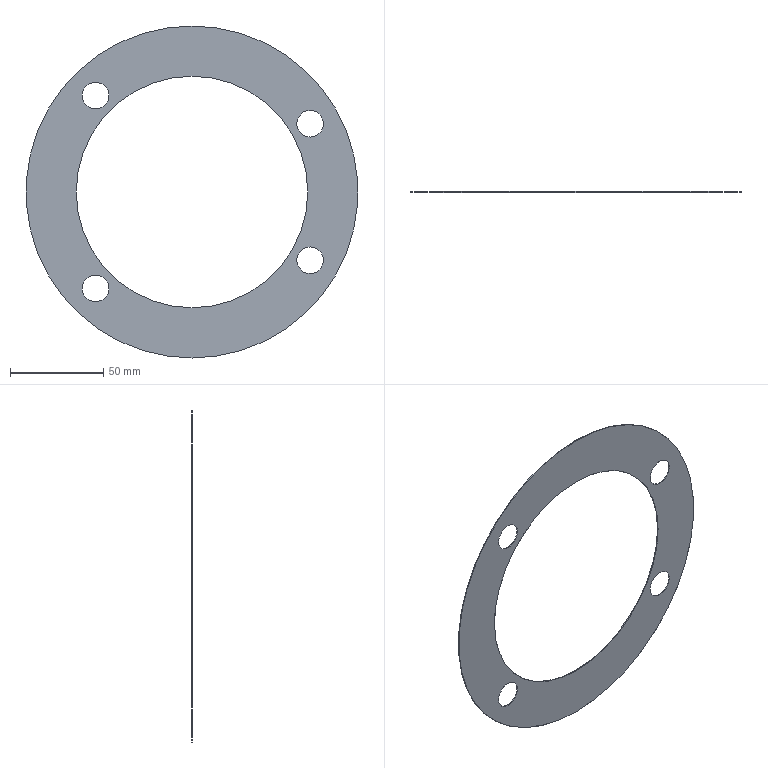Part | SolidWorks | features 3DProfileFeature 1, Extrusion 1, HoleWzd 1, MirrorPattern 1 | 1 solid | 14 faces | box 177.8 x 0.381 x 177.8 mm | volume 4618 mm3 | cylinder 12 | plane 2 | commonest cylinder face diameters 14.287 x8 123.95 x2 177.8 x2
STEP:
#1=CARTESIAN_POINT('',(-51.638,0.,44.496));
#2=VERTEX_POINT('',#1);
#3=CARTESIAN_POINT('',(-51.638,0.,58.784));
#4=VERTEX_POINT('',#3);
#5=CARTESIAN_POINT('',(-51.638,0.,51.64));
#6=DIRECTION('',(0.,1.,0.));
#7=DIRECTION('',(0.,0.,1.));
#8=AXIS2_PLACEMENT_3D('',#5,#6,#7);
#9=CIRCLE('',#8,7.144);
#10=EDGE_CURVE('',#2,#4,#9,.T.);
#11=ORIENTED_EDGE('',*,*,#10,.F.);
#12=CARTESIAN_POINT('',(-51.638,0.381,44.496));
#13=VERTEX_POINT('',#12);
#14=CARTESIAN_POINT('',(-51.638,0.381,44.496));
#15=DIRECTION('',(0.,1.,0.));
#16=VECTOR('',#15,1000.);
#17=LINE('',#14,#16);
#18=EDGE_CURVE('',#2,#13,#17,.T.);
#19=ORIENTED_EDGE('',*,*,#18,.T.);
#20=CARTESIAN_POINT('',(-51.638,0.381,58.784));
#21=VERTEX_POINT('',#20);
#22=CARTESIAN_POINT('',(-51.638,0.381,51.64));
#23=DIRECTION('',(0.,1.,0.));
#24=DIRECTION('',(0.,0.,1.));
#25=AXIS2_PLACEMENT_3D('',#22,#23,#24);
#26=CIRCLE('',#25,7.144);
#27=EDGE_CURVE('',#13,#21,#26,.T.);
#28=ORIENTED_EDGE('',*,*,#27,.T.);
#29=CARTESIAN_POINT('',(-51.638,0.381,58.784));
#30=DIRECTION('',(0.,1.,0.));
#31=VECTOR('',#30,1000.);
#32=LINE('',#29,#31);
#33=EDGE_CURVE('',#4,#21,#32,.T.);
#34=ORIENTED_EDGE('',*,*,#33,.F.);
#35=EDGE_LOOP('',(#11,#19,#28,#34));
#36=FACE_OUTER_BOUND('',#35,.T.);
#37=CARTESIAN_POINT('',(-51.638,0.381,51.64));
#38=DIRECTION('',(0.,1.,0.));
#39=DIRECTION('',(0.,0.,1.));
#40=AXIS2_PLACEMENT_3D('',#37,#38,#39);
#41=CYLINDRICAL_SURFACE('',#40,7.144);
#42=ADVANCED_FACE('',(#36),#41,.F.);
#43=CARTESIAN_POINT('',(63.246,0.,-43.674));
#44=VERTEX_POINT('',#43);
#45=CARTESIAN_POINT('',(63.246,0.,-29.386));
#46=VERTEX_POINT('',#45);
#47=CARTESIAN_POINT('',(63.246,0.,-36.53));
#48=DIRECTION('',(0.,1.,0.));
#49=DIRECTION('',(0.,0.,1.));
#50=AXIS2_PLACEMENT_3D('',#47,#48,#49);
#51=CIRCLE('',#50,7.144);
#52=EDGE_CURVE('',#44,#46,#51,.T.);
#53=ORIENTED_EDGE('',*,*,#52,.F.);
#54=CARTESIAN_POINT('',(63.246,0.381,-43.674));
#55=VERTEX_POINT('',#54);
#56=CARTESIAN_POINT('',(63.246,0.381,-43.674));
#57=DIRECTION('',(0.,1.,0.));
#58=VECTOR('',#57,1000.);
#59=LINE('',#56,#58);
#60=EDGE_CURVE('',#44,#55,#59,.T.);
#61=ORIENTED_EDGE('',*,*,#60,.T.);
#62=CARTESIAN_POINT('',(63.246,0.381,-29.386));
#63=VERTEX_POINT('',#62);
#64=CARTESIAN_POINT('',(63.246,0.381,-36.53));
#65=DIRECTION('',(0.,1.,0.));
#66=DIRECTION('',(0.,0.,1.));
#67=AXIS2_PLACEMENT_3D('',#64,#65,#66);
#68=CIRCLE('',#67,7.144);
#69=EDGE_CURVE('',#55,#63,#68,.T.);
#70=ORIENTED_EDGE('',*,*,#69,.T.);
#71=CARTESIAN_POINT('',(63.246,0.381,-29.386));
#72=DIRECTION('',(0.,1.,0.));
#73=VECTOR('',#72,1000.);
#74=LINE('',#71,#73);
#75=EDGE_CURVE('',#46,#63,#74,.T.);
#76=ORIENTED_EDGE('',*,*,#75,.F.);
#77=EDGE_LOOP('',(#53,#61,#70,#76));
#78=FACE_OUTER_BOUND('',#77,.T.);
#79=CARTESIAN_POINT('',(63.246,0.381,-36.53));
#80=DIRECTION('',(0.,1.,0.));
#81=DIRECTION('',(0.,0.,1.));
#82=AXIS2_PLACEMENT_3D('',#79,#80,#81);
#83=CYLINDRICAL_SURFACE('',#82,7.144);
#84=ADVANCED_FACE('',(#78),#83,.F.);
#85=CARTESIAN_POINT('',(-51.638,0.,-58.784));
#86=VERTEX_POINT('',#85);
#87=CARTESIAN_POINT('',(-51.638,0.,-44.496));
#88=VERTEX_POINT('',#87);
#89=CARTESIAN_POINT('',(-51.638,0.,-51.64));
#90=DIRECTION('',(0.,1.,0.));
#91=DIRECTION('',(0.,0.,1.));
#92=AXIS2_PLACEMENT_3D('',#89,#90,#91);
#93=CIRCLE('',#92,7.144);
#94=EDGE_CURVE('',#86,#88,#93,.T.);
#95=ORIENTED_EDGE('',*,*,#94,.F.);
#96=CARTESIAN_POINT('',(-51.638,0.381,-58.784));
#97=VERTEX_POINT('',#96);
#98=CARTESIAN_POINT('',(-51.638,0.381,-58.784));
#99=DIRECTION('',(0.,1.,0.));
#100=VECTOR('',#99,1000.);
#101=LINE('',#98,#100);
#102=EDGE_CURVE('',#86,#97,#101,.T.);
#103=ORIENTED_EDGE('',*,*,#102,.T.);
#104=CARTESIAN_POINT('',(-51.638,0.381,-44.496));
#105=VERTEX_POINT('',#104);
#106=CARTESIAN_POINT('',(-51.638,0.381,-51.64));
#107=DIRECTION('',(0.,1.,0.));
#108=DIRECTION('',(0.,0.,1.));
#109=AXIS2_PLACEMENT_3D('',#106,#107,#108);
#110=CIRCLE('',#109,7.144);
#111=EDGE_CURVE('',#97,#105,#110,.T.);
#112=ORIENTED_EDGE('',*,*,#111,.T.);
#113=CARTESIAN_POINT('',(-51.638,0.381,-44.496));
#114=DIRECTION('',(0.,1.,0.));
#115=VECTOR('',#114,1000.);
#116=LINE('',#113,#115);
#117=EDGE_CURVE('',#88,#105,#116,.T.);
#118=ORIENTED_EDGE('',*,*,#117,.F.);
#119=EDGE_LOOP('',(#95,#103,#112,#118));
#120=FACE_OUTER_BOUND('',#119,.T.);
#121=CARTESIAN_POINT('',(-51.638,0.381,-51.64));
#122=DIRECTION('',(0.,1.,0.));
#123=DIRECTION('',(0.,0.,1.));
#124=AXIS2_PLACEMENT_3D('',#121,#122,#123);
#125=CYLINDRICAL_SURFACE('',#124,7.144);
#126=ADVANCED_FACE('',(#120),#125,.F.);
#127=CARTESIAN_POINT('',(63.246,0.,29.386));
#128=VERTEX_POINT('',#127);
#129=CARTESIAN_POINT('',(63.246,0.,43.674));
#130=VERTEX_POINT('',#129);
#131=CARTESIAN_POINT('',(63.246,0.,36.53));
#132=DIRECTION('',(0.,1.,0.));
#133=DIRECTION('',(0.,0.,1.));
#134=AXIS2_PLACEMENT_3D('',#131,#132,#133);
#135=CIRCLE('',#134,7.144);
#136=EDGE_CURVE('',#128,#130,#135,.T.);
#137=ORIENTED_EDGE('',*,*,#136,.F.);
#138=CARTESIAN_POINT('',(63.246,0.381,29.386));
#139=VERTEX_POINT('',#138);
#140=CARTESIAN_POINT('',(63.246,0.381,29.386));
#141=DIRECTION('',(0.,1.,0.));
#142=VECTOR('',#141,1000.);
#143=LINE('',#140,#142);
#144=EDGE_CURVE('',#128,#139,#143,.T.);
#145=ORIENTED_EDGE('',*,*,#144,.T.);
#146=CARTESIAN_POINT('',(63.246,0.381,43.674));
#147=VERTEX_POINT('',#146);
#148=CARTESIAN_POINT('',(63.246,0.381,36.53));
#149=DIRECTION('',(0.,1.,0.));
#150=DIRECTION('',(0.,0.,1.));
#151=AXIS2_PLACEMENT_3D('',#148,#149,#150);
#152=CIRCLE('',#151,7.144);
#153=EDGE_CURVE('',#139,#147,#152,.T.);
#154=ORIENTED_EDGE('',*,*,#153,.T.);
#155=CARTESIAN_POINT('',(63.246,0.381,43.674));
#156=DIRECTION('',(0.,1.,0.));
#157=VECTOR('',#156,1000.);
#158=LINE('',#155,#157);
#159=EDGE_CURVE('',#130,#147,#158,.T.);
#160=ORIENTED_EDGE('',*,*,#159,.F.);
#161=EDGE_LOOP('',(#137,#145,#154,#160));
#162=FACE_OUTER_BOUND('',#161,.T.);
#163=CARTESIAN_POINT('',(63.246,0.381,36.53));
#164=DIRECTION('',(0.,1.,0.));
#165=DIRECTION('',(0.,0.,1.));
#166=AXIS2_PLACEMENT_3D('',#163,#164,#165);
#167=CYLINDRICAL_SURFACE('',#166,7.144);
#168=ADVANCED_FACE('',(#162),#167,.F.);
#169=CARTESIAN_POINT('',(0.,0.381,-61.975));
#170=VERTEX_POINT('',#169);
#171=CARTESIAN_POINT('',(0.,0.381,61.975));
#172=VERTEX_POINT('',#171);
#173=CARTESIAN_POINT('',(0.,0.381,0.));
#174=DIRECTION('',(0.,1.,0.));
#175=DIRECTION('',(0.,0.,1.));
#176=AXIS2_PLACEMENT_3D('',#173,#174,#175);
#177=CIRCLE('',#176,61.975);
#178=EDGE_CURVE('',#170,#172,#177,.T.);
#179=ORIENTED_EDGE('',*,*,#178,.T.);
#180=CARTESIAN_POINT('',(0.,0.,61.975));
#181=VERTEX_POINT('',#180);
#182=CARTESIAN_POINT('',(0.,0.381,61.975));
#183=DIRECTION('',(0.,-1.,0.));
#184=VECTOR('',#183,1000.);
#185=LINE('',#182,#184);
#186=EDGE_CURVE('',#172,#181,#185,.T.);
#187=ORIENTED_EDGE('',*,*,#186,.T.);
#188=CARTESIAN_POINT('',(0.,0.,-61.975));
#189=VERTEX_POINT('',#188);
#190=CARTESIAN_POINT('',(0.,0.,0.));
#191=DIRECTION('',(0.,1.,0.));
#192=DIRECTION('',(0.,0.,1.));
#193=AXIS2_PLACEMENT_3D('',#190,#191,#192);
#194=CIRCLE('',#193,61.975);
#195=EDGE_CURVE('',#189,#181,#194,.T.);
#196=ORIENTED_EDGE('',*,*,#195,.F.);
#197=CARTESIAN_POINT('',(0.,0.381,-61.975));
#198=DIRECTION('',(0.,-1.,0.));
#199=VECTOR('',#198,1000.);
#200=LINE('',#197,#199);
#201=EDGE_CURVE('',#170,#189,#200,.T.);
#202=ORIENTED_EDGE('',*,*,#201,.F.);
#203=EDGE_LOOP('',(#179,#187,#196,#202));
#204=FACE_OUTER_BOUND('',#203,.T.);
#205=CARTESIAN_POINT('',(0.,0.381,0.));
#206=DIRECTION('',(0.,-1.,0.));
#207=DIRECTION('',(0.,0.,-1.));
#208=AXIS2_PLACEMENT_3D('',#205,#206,#207);
#209=CYLINDRICAL_SURFACE('',#208,61.975);
#210=ADVANCED_FACE('',(#204),#209,.F.);
#211=CARTESIAN_POINT('',(0.,0.381,88.9));
#212=VERTEX_POINT('',#211);
#213=CARTESIAN_POINT('',(0.,0.381,-88.9));
#214=VERTEX_POINT('',#213);
#215=CARTESIAN_POINT('',(0.,0.381,0.));
#216=DIRECTION('',(0.,1.,0.));
#217=DIRECTION('',(0.,0.,1.));
#218=AXIS2_PLACEMENT_3D('',#215,#216,#217);
#219=CIRCLE('',#218,88.9);
#220=EDGE_CURVE('',#212,#214,#219,.T.);
#221=ORIENTED_EDGE('',*,*,#220,.F.);
#222=CARTESIAN_POINT('',(0.,0.,88.9));
#223=VERTEX_POINT('',#222);
#224=CARTESIAN_POINT('',(0.,0.381,88.9));
#225=DIRECTION('',(0.,-1.,0.));
#226=VECTOR('',#225,1000.);
#227=LINE('',#224,#226);
#228=EDGE_CURVE('',#212,#223,#227,.T.);
#229=ORIENTED_EDGE('',*,*,#228,.T.);
#230=CARTESIAN_POINT('',(0.,0.,-88.9));
#231=VERTEX_POINT('',#230);
#232=CARTESIAN_POINT('',(0.,0.,0.));
#233=DIRECTION('',(0.,1.,0.));
#234=DIRECTION('',(0.,0.,1.));
#235=AXIS2_PLACEMENT_3D('',#232,#233,#234);
#236=CIRCLE('',#235,88.9);
#237=EDGE_CURVE('',#223,#231,#236,.T.);
#238=ORIENTED_EDGE('',*,*,#237,.T.);
#239=CARTESIAN_POINT('',(0.,0.381,-88.9));
#240=DIRECTION('',(0.,-1.,0.));
#241=VECTOR('',#240,1000.);
#242=LINE('',#239,#241);
#243=EDGE_CURVE('',#214,#231,#242,.T.);
#244=ORIENTED_EDGE('',*,*,#243,.F.);
#245=EDGE_LOOP('',(#221,#229,#238,#244));
#246=FACE_OUTER_BOUND('',#245,.T.);
#247=CARTESIAN_POINT('',(0.,0.381,0.));
#248=DIRECTION('',(0.,-1.,0.));
#249=DIRECTION('',(0.,0.,-1.));
#250=AXIS2_PLACEMENT_3D('',#247,#248,#249);
#251=CYLINDRICAL_SURFACE('',#250,88.9);
#252=ADVANCED_FACE('',(#246),#251,.T.);
#253=CARTESIAN_POINT('',(-51.638,0.381,51.64));
#254=DIRECTION('',(0.,1.,0.));
#255=DIRECTION('',(0.,0.,1.));
#256=AXIS2_PLACEMENT_3D('',#253,#254,#255);
#257=CIRCLE('',#256,7.144);
#258=EDGE_CURVE('',#21,#13,#257,.T.);
#259=ORIENTED_EDGE('',*,*,#258,.F.);
#260=ORIENTED_EDGE('',*,*,#27,.F.);
#261=EDGE_LOOP('',(#259,#260));
#262=FACE_BOUND('',#261,.T.);
#263=CARTESIAN_POINT('',(63.246,0.381,-36.53));
#264=DIRECTION('',(0.,1.,0.));
#265=DIRECTION('',(0.,0.,1.));
#266=AXIS2_PLACEMENT_3D('',#263,#264,#265);
#267=CIRCLE('',#266,7.144);
#268=EDGE_CURVE('',#63,#55,#267,.T.);
#269=ORIENTED_EDGE('',*,*,#268,.F.);
#270=ORIENTED_EDGE('',*,*,#69,.F.);
#271=EDGE_LOOP('',(#269,#270));
#272=FACE_BOUND('',#271,.T.);
#273=CARTESIAN_POINT('',(-51.638,0.381,-51.64));
#274=DIRECTION('',(0.,1.,0.));
#275=DIRECTION('',(0.,0.,1.));
#276=AXIS2_PLACEMENT_3D('',#273,#274,#275);
#277=CIRCLE('',#276,7.144);
#278=EDGE_CURVE('',#105,#97,#277,.T.);
#279=ORIENTED_EDGE('',*,*,#278,.F.);
#280=ORIENTED_EDGE('',*,*,#111,.F.);
#281=EDGE_LOOP('',(#279,#280));
#282=FACE_BOUND('',#281,.T.);
#283=CARTESIAN_POINT('',(63.246,0.381,36.53));
#284=DIRECTION('',(0.,1.,0.));
#285=DIRECTION('',(0.,0.,1.));
#286=AXIS2_PLACEMENT_3D('',#283,#284,#285);
#287=CIRCLE('',#286,7.144);
#288=EDGE_CURVE('',#147,#139,#287,.T.);
#289=ORIENTED_EDGE('',*,*,#288,.F.);
#290=ORIENTED_EDGE('',*,*,#153,.F.);
#291=EDGE_LOOP('',(#289,#290));
#292=FACE_BOUND('',#291,.T.);
#293=CARTESIAN_POINT('',(0.,0.381,0.));
#294=DIRECTION('',(0.,1.,0.));
#295=DIRECTION('',(0.,0.,1.));
#296=AXIS2_PLACEMENT_3D('',#293,#294,#295);
#297=CIRCLE('',#296,88.9);
#298=EDGE_CURVE('',#214,#212,#297,.T.);
#299=ORIENTED_EDGE('',*,*,#298,.T.);
#300=ORIENTED_EDGE('',*,*,#220,.T.);
#301=EDGE_LOOP('',(#299,#300));
#302=FACE_OUTER_BOUND('',#301,.T.);
#303=ORIENTED_EDGE('',*,*,#178,.F.);
#304=CARTESIAN_POINT('',(0.,0.381,0.));
#305=DIRECTION('',(0.,1.,0.));
#306=DIRECTION('',(0.,0.,1.));
#307=AXIS2_PLACEMENT_3D('',#304,#305,#306);
#308=CIRCLE('',#307,61.975);
#309=EDGE_CURVE('',#172,#170,#308,.T.);
#310=ORIENTED_EDGE('',*,*,#309,.F.);
#311=EDGE_LOOP('',(#303,#310));
#312=FACE_BOUND('',#311,.T.);
#313=CARTESIAN_POINT('',(0.,0.381,0.));
#314=DIRECTION('',(0.,1.,0.));
#315=DIRECTION('',(0.,0.,1.));
#316=AXIS2_PLACEMENT_3D('',#313,#314,#315);
#317=PLANE('',#316);
#318=ADVANCED_FACE('',(#262,#272,#282,#292,#302,#312),#317,.T.);
#319=CARTESIAN_POINT('',(-51.638,0.,51.64));
#320=DIRECTION('',(0.,1.,0.));
#321=DIRECTION('',(0.,0.,1.));
#322=AXIS2_PLACEMENT_3D('',#319,#320,#321);
#323=CIRCLE('',#322,7.144);
#324=EDGE_CURVE('',#4,#2,#323,.T.);
#325=ORIENTED_EDGE('',*,*,#324,.T.);
#326=ORIENTED_EDGE('',*,*,#10,.T.);
#327=EDGE_LOOP('',(#325,#326));
#328=FACE_BOUND('',#327,.T.);
#329=CARTESIAN_POINT('',(63.246,0.,-36.53));
#330=DIRECTION('',(0.,1.,0.));
#331=DIRECTION('',(0.,0.,1.));
#332=AXIS2_PLACEMENT_3D('',#329,#330,#331);
#333=CIRCLE('',#332,7.144);
#334=EDGE_CURVE('',#46,#44,#333,.T.);
#335=ORIENTED_EDGE('',*,*,#334,.T.);
#336=ORIENTED_EDGE('',*,*,#52,.T.);
#337=EDGE_LOOP('',(#335,#336));
#338=FACE_BOUND('',#337,.T.);
#339=CARTESIAN_POINT('',(-51.638,0.,-51.64));
#340=DIRECTION('',(0.,1.,0.));
#341=DIRECTION('',(0.,0.,1.));
#342=AXIS2_PLACEMENT_3D('',#339,#340,#341);
#343=CIRCLE('',#342,7.144);
#344=EDGE_CURVE('',#88,#86,#343,.T.);
#345=ORIENTED_EDGE('',*,*,#344,.T.);
#346=ORIENTED_EDGE('',*,*,#94,.T.);
#347=EDGE_LOOP('',(#345,#346));
#348=FACE_BOUND('',#347,.T.);
#349=CARTESIAN_POINT('',(63.246,0.,36.53));
#350=DIRECTION('',(0.,1.,0.));
#351=DIRECTION('',(0.,0.,1.));
#352=AXIS2_PLACEMENT_3D('',#349,#350,#351);
#353=CIRCLE('',#352,7.144);
#354=EDGE_CURVE('',#130,#128,#353,.T.);
#355=ORIENTED_EDGE('',*,*,#354,.T.);
#356=ORIENTED_EDGE('',*,*,#136,.T.);
#357=EDGE_LOOP('',(#355,#356));
#358=FACE_BOUND('',#357,.T.);
#359=CARTESIAN_POINT('',(0.,0.,0.));
#360=DIRECTION('',(0.,1.,0.));
#361=DIRECTION('',(0.,0.,1.));
#362=AXIS2_PLACEMENT_3D('',#359,#360,#361);
#363=CIRCLE('',#362,88.9);
#364=EDGE_CURVE('',#231,#223,#363,.T.);
#365=ORIENTED_EDGE('',*,*,#364,.F.);
#366=ORIENTED_EDGE('',*,*,#237,.F.);
#367=EDGE_LOOP('',(#365,#366));
#368=FACE_OUTER_BOUND('',#367,.T.);
#369=ORIENTED_EDGE('',*,*,#195,.T.);
#370=CARTESIAN_POINT('',(0.,0.,0.));
#371=DIRECTION('',(0.,1.,0.));
#372=DIRECTION('',(0.,0.,1.));
#373=AXIS2_PLACEMENT_3D('',#370,#371,#372);
#374=CIRCLE('',#373,61.975);
#375=EDGE_CURVE('',#181,#189,#374,.T.);
#376=ORIENTED_EDGE('',*,*,#375,.T.);
#377=EDGE_LOOP('',(#369,#376));
#378=FACE_BOUND('',#377,.T.);
#379=CARTESIAN_POINT('',(0.,0.,0.));
#380=DIRECTION('',(0.,1.,0.));
#381=DIRECTION('',(0.,0.,1.));
#382=AXIS2_PLACEMENT_3D('',#379,#380,#381);
#383=PLANE('',#382);
#384=ADVANCED_FACE('',(#328,#338,#348,#358,#368,#378),#383,.F.);
#385=ORIENTED_EDGE('',*,*,#228,.F.);
#386=ORIENTED_EDGE('',*,*,#298,.F.);
#387=ORIENTED_EDGE('',*,*,#243,.T.);
#388=ORIENTED_EDGE('',*,*,#364,.T.);
#389=EDGE_LOOP('',(#385,#386,#387,#388));
#390=FACE_OUTER_BOUND('',#389,.T.);
#391=CARTESIAN_POINT('',(0.,0.381,0.));
#392=DIRECTION('',(0.,-1.,0.));
#393=DIRECTION('',(0.,0.,-1.));
#394=AXIS2_PLACEMENT_3D('',#391,#392,#393);
#395=CYLINDRICAL_SURFACE('',#394,88.9);
#396=ADVANCED_FACE('',(#390),#395,.T.);
#397=ORIENTED_EDGE('',*,*,#186,.F.);
#398=ORIENTED_EDGE('',*,*,#309,.T.);
#399=ORIENTED_EDGE('',*,*,#201,.T.);
#400=ORIENTED_EDGE('',*,*,#375,.F.);
#401=EDGE_LOOP('',(#397,#398,#399,#400));
#402=FACE_OUTER_BOUND('',#401,.T.);
#403=CARTESIAN_POINT('',(0.,0.381,0.));
#404=DIRECTION('',(0.,-1.,0.));
#405=DIRECTION('',(0.,0.,-1.));
#406=AXIS2_PLACEMENT_3D('',#403,#404,#405);
#407=CYLINDRICAL_SURFACE('',#406,61.975);
#408=ADVANCED_FACE('',(#402),#407,.F.);
#409=ORIENTED_EDGE('',*,*,#144,.F.);
#410=ORIENTED_EDGE('',*,*,#354,.F.);
#411=ORIENTED_EDGE('',*,*,#159,.T.);
#412=ORIENTED_EDGE('',*,*,#288,.T.);
#413=EDGE_LOOP('',(#409,#410,#411,#412));
#414=FACE_OUTER_BOUND('',#413,.T.);
#415=CARTESIAN_POINT('',(63.246,0.381,36.53));
#416=DIRECTION('',(0.,1.,0.));
#417=DIRECTION('',(0.,0.,1.));
#418=AXIS2_PLACEMENT_3D('',#415,#416,#417);
#419=CYLINDRICAL_SURFACE('',#418,7.144);
#420=ADVANCED_FACE('',(#414),#419,.F.);
#421=ORIENTED_EDGE('',*,*,#102,.F.);
#422=ORIENTED_EDGE('',*,*,#344,.F.);
#423=ORIENTED_EDGE('',*,*,#117,.T.);
#424=ORIENTED_EDGE('',*,*,#278,.T.);
#425=EDGE_LOOP('',(#421,#422,#423,#424));
#426=FACE_OUTER_BOUND('',#425,.T.);
#427=CARTESIAN_POINT('',(-51.638,0.381,-51.64));
#428=DIRECTION('',(0.,1.,0.));
#429=DIRECTION('',(0.,0.,1.));
#430=AXIS2_PLACEMENT_3D('',#427,#428,#429);
#431=CYLINDRICAL_SURFACE('',#430,7.144);
#432=ADVANCED_FACE('',(#426),#431,.F.);
#433=ORIENTED_EDGE('',*,*,#60,.F.);
#434=ORIENTED_EDGE('',*,*,#334,.F.);
#435=ORIENTED_EDGE('',*,*,#75,.T.);
#436=ORIENTED_EDGE('',*,*,#268,.T.);
#437=EDGE_LOOP('',(#433,#434,#435,#436));
#438=FACE_OUTER_BOUND('',#437,.T.);
#439=CARTESIAN_POINT('',(63.246,0.381,-36.53));
#440=DIRECTION('',(0.,1.,0.));
#441=DIRECTION('',(0.,0.,1.));
#442=AXIS2_PLACEMENT_3D('',#439,#440,#441);
#443=CYLINDRICAL_SURFACE('',#442,7.144);
#444=ADVANCED_FACE('',(#438),#443,.F.);
#445=ORIENTED_EDGE('',*,*,#18,.F.);
#446=ORIENTED_EDGE('',*,*,#324,.F.);
#447=ORIENTED_EDGE('',*,*,#33,.T.);
#448=ORIENTED_EDGE('',*,*,#258,.T.);
#449=EDGE_LOOP('',(#445,#446,#447,#448));
#450=FACE_OUTER_BOUND('',#449,.T.);
#451=CARTESIAN_POINT('',(-51.638,0.381,51.64));
#452=DIRECTION('',(0.,1.,0.));
#453=DIRECTION('',(0.,0.,1.));
#454=AXIS2_PLACEMENT_3D('',#451,#452,#453);
#455=CYLINDRICAL_SURFACE('',#454,7.144);
#456=ADVANCED_FACE('',(#450),#455,.F.);
#457=CLOSED_SHELL('',(#42,#84,#126,#168,#210,#252,#318,#384,#396,#408,#420,#432,#444,#456));
#458=MANIFOLD_SOLID_BREP('',#457);
#459=CARTESIAN_POINT('',(0.,0.,0.));
#460=DIRECTION('',(0.,0.,1.));
#461=DIRECTION('',(1.,0.,0.));
#462=AXIS2_PLACEMENT_3D('',#459,#460,#461);
#463=(LENGTH_UNIT()NAMED_UNIT(*)SI_UNIT(.MILLI.,.METRE.));
#464=UNCERTAINTY_MEASURE_WITH_UNIT(LENGTH_MEASURE(0.00001),#463,'','');
#465=(NAMED_UNIT(*)PLANE_ANGLE_UNIT()SI_UNIT($,.RADIAN.));
#466=(NAMED_UNIT(*)SI_UNIT($,.STERADIAN.)SOLID_ANGLE_UNIT());
#467=(GEOMETRIC_REPRESENTATION_CONTEXT(3)GLOBAL_UNCERTAINTY_ASSIGNED_CONTEXT((#464))GLOBAL_UNIT_ASSIGNED_CONTEXT((#463,#465,#466))REPRESENTATION_CONTEXT('',''));
#468=ADVANCED_BREP_SHAPE_REPRESENTATION('',(#458,#462),#467);